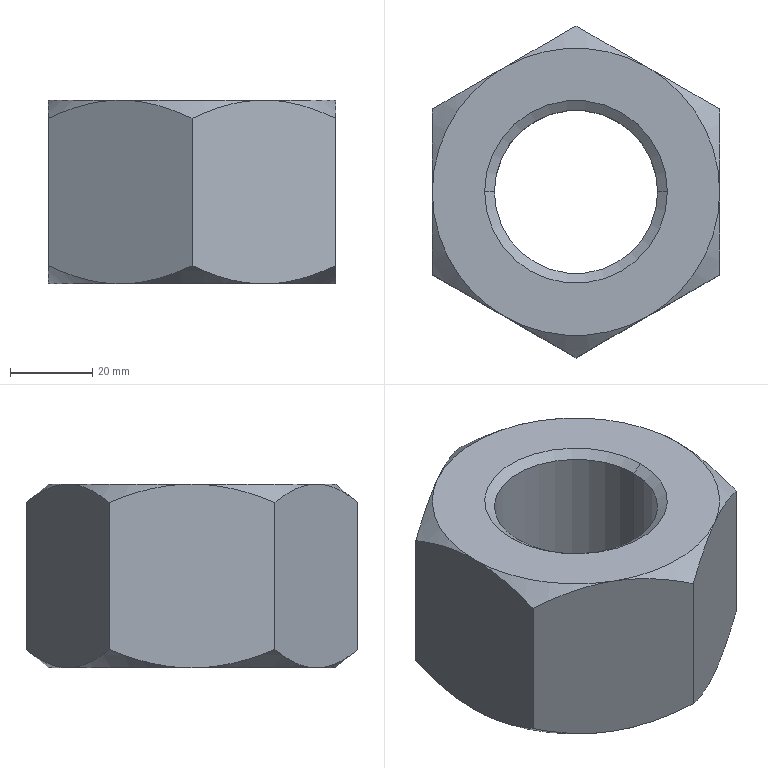Part | SolidWorks | features RevCut 4, Extrusion 1, LPattern 1 | 1 solid | 28 faces | box 69.85 x 80.656 x 44.679 mm | volume 131935 mm3 | cone 16 | plane 8 | cylinder 4 | commonest cylinder face diameters 39.688 x2 44.45 x2
STEP:
#1=CARTESIAN_POINT('',(0.875,0.,-1.759));
#2=VERTEX_POINT('',#1);
#3=CARTESIAN_POINT('',(-0.875,0.,-1.759));
#4=VERTEX_POINT('',#3);
#5=CARTESIAN_POINT('',(0.,0.,-1.759));
#6=DIRECTION('',(0.,0.,-1.));
#7=DIRECTION('',(1.,0.,0.));
#8=AXIS2_PLACEMENT_3D('',#5,#6,#7);
#9=CIRCLE('',#8,0.875);
#10=EDGE_CURVE('',#2,#4,#9,.T.);
#11=ORIENTED_EDGE('',*,*,#10,.T.);
#12=CARTESIAN_POINT('',(-0.875,0.,-1.758));
#13=VERTEX_POINT('',#12);
#14=CARTESIAN_POINT('',(-0.875,0.,-0.9857));
#15=DIRECTION('',(0.,0.,1.));
#16=VECTOR('',#15,39.37);
#17=LINE('',#14,#16);
#18=EDGE_CURVE('',#4,#13,#17,.T.);
#19=ORIENTED_EDGE('',*,*,#18,.T.);
#20=CARTESIAN_POINT('',(0.875,0.,-1.758));
#21=VERTEX_POINT('',#20);
#22=CARTESIAN_POINT('',(0.,0.,-1.758));
#23=DIRECTION('',(0.,0.,1.));
#24=DIRECTION('',(1.,0.,0.));
#25=AXIS2_PLACEMENT_3D('',#22,#23,#24);
#26=CIRCLE('',#25,0.875);
#27=EDGE_CURVE('',#13,#21,#26,.T.);
#28=ORIENTED_EDGE('',*,*,#27,.T.);
#29=CARTESIAN_POINT('',(0.875,0.,-0.9857));
#30=DIRECTION('',(0.,0.,1.));
#31=VECTOR('',#30,39.37);
#32=LINE('',#29,#31);
#33=EDGE_CURVE('',#2,#21,#32,.T.);
#34=ORIENTED_EDGE('',*,*,#33,.F.);
#35=EDGE_LOOP('',(#11,#19,#28,#34));
#36=FACE_OUTER_BOUND('',#35,.T.);
#37=CARTESIAN_POINT('',(0.,0.,-0.9857));
#38=DIRECTION('',(0.,0.,1.));
#39=DIRECTION('',(1.,0.,0.));
#40=AXIS2_PLACEMENT_3D('',#37,#38,#39);
#41=CYLINDRICAL_SURFACE('',#40,0.875);
#42=ADVANCED_FACE('',(#36),#41,.F.);
#43=CARTESIAN_POINT('',(-0.7812,0.,-1.692));
#44=VERTEX_POINT('',#43);
#45=CARTESIAN_POINT('',(0.7812,0.,-1.692));
#46=VERTEX_POINT('',#45);
#47=CARTESIAN_POINT('',(0.,0.,-1.692));
#48=DIRECTION('',(0.,0.,1.));
#49=DIRECTION('',(-1.,0.,0.));
#50=AXIS2_PLACEMENT_3D('',#47,#48,#49);
#51=CIRCLE('',#50,0.7812);
#52=EDGE_CURVE('',#44,#46,#51,.T.);
#53=ORIENTED_EDGE('',*,*,#52,.T.);
#54=CARTESIAN_POINT('',(0.875,0.,-1.758));
#55=DIRECTION('',(0.8192,0.,-0.5736));
#56=VECTOR('',#55,39.37);
#57=LINE('',#54,#56);
#58=EDGE_CURVE('',#46,#21,#57,.T.);
#59=ORIENTED_EDGE('',*,*,#58,.T.);
#60=ORIENTED_EDGE('',*,*,#27,.F.);
#61=CARTESIAN_POINT('',(-0.875,0.,-1.758));
#62=DIRECTION('',(-0.8192,0.,-0.5736));
#63=VECTOR('',#62,39.37);
#64=LINE('',#61,#63);
#65=EDGE_CURVE('',#44,#13,#64,.T.);
#66=ORIENTED_EDGE('',*,*,#65,.F.);
#67=EDGE_LOOP('',(#53,#59,#60,#66));
#68=FACE_OUTER_BOUND('',#67,.T.);
#69=CARTESIAN_POINT('',(0.,0.,-1.758));
#70=DIRECTION('',(0.,0.,-1.));
#71=DIRECTION('',(-1.,0.,0.));
#72=AXIS2_PLACEMENT_3D('',#69,#70,#71);
#73=CONICAL_SURFACE('',#72,0.875,0.9599);
#74=ADVANCED_FACE('',(#68),#73,.F.);
#75=CARTESIAN_POINT('',(0.7812,0.,-0.06564));
#76=VERTEX_POINT('',#75);
#77=CARTESIAN_POINT('',(-0.7812,0.,-0.06564));
#78=VERTEX_POINT('',#77);
#79=CARTESIAN_POINT('',(0.,0.,-0.06564));
#80=DIRECTION('',(0.,0.,-1.));
#81=DIRECTION('',(1.,0.,0.));
#82=AXIS2_PLACEMENT_3D('',#79,#80,#81);
#83=CIRCLE('',#82,0.7812);
#84=EDGE_CURVE('',#76,#78,#83,.T.);
#85=ORIENTED_EDGE('',*,*,#84,.T.);
#86=CARTESIAN_POINT('',(-0.875,0.,0.));
#87=VERTEX_POINT('',#86);
#88=CARTESIAN_POINT('',(-0.7719,0.,-0.07221));
#89=DIRECTION('',(-0.8192,0.,0.5736));
#90=VECTOR('',#89,39.37);
#91=LINE('',#88,#90);
#92=EDGE_CURVE('',#78,#87,#91,.T.);
#93=ORIENTED_EDGE('',*,*,#92,.T.);
#94=CARTESIAN_POINT('',(0.875,0.,0.));
#95=VERTEX_POINT('',#94);
#96=CARTESIAN_POINT('',(0.,0.,0.));
#97=DIRECTION('',(0.,0.,1.));
#98=DIRECTION('',(1.,0.,0.));
#99=AXIS2_PLACEMENT_3D('',#96,#97,#98);
#100=CIRCLE('',#99,0.875);
#101=EDGE_CURVE('',#87,#95,#100,.T.);
#102=ORIENTED_EDGE('',*,*,#101,.T.);
#103=CARTESIAN_POINT('',(0.7719,0.,-0.07221));
#104=DIRECTION('',(0.8192,0.,0.5736));
#105=VECTOR('',#104,39.37);
#106=LINE('',#103,#105);
#107=EDGE_CURVE('',#76,#95,#106,.T.);
#108=ORIENTED_EDGE('',*,*,#107,.F.);
#109=EDGE_LOOP('',(#85,#93,#102,#108));
#110=FACE_OUTER_BOUND('',#109,.T.);
#111=CARTESIAN_POINT('',(0.,0.,-0.07221));
#112=DIRECTION('',(0.,0.,1.));
#113=DIRECTION('',(1.,0.,0.));
#114=AXIS2_PLACEMENT_3D('',#111,#112,#113);
#115=CONICAL_SURFACE('',#114,0.7719,0.9599);
#116=ADVANCED_FACE('',(#110),#115,.F.);
#117=ORIENTED_EDGE('',*,*,#52,.F.);
#118=CARTESIAN_POINT('',(-0.7812,0.,-1.759));
#119=DIRECTION('',(0.,0.,1.));
#120=VECTOR('',#119,39.37);
#121=LINE('',#118,#120);
#122=EDGE_CURVE('',#44,#78,#121,.T.);
#123=ORIENTED_EDGE('',*,*,#122,.T.);
#124=ORIENTED_EDGE('',*,*,#84,.F.);
#125=CARTESIAN_POINT('',(0.7812,0.,-1.759));
#126=DIRECTION('',(0.,0.,1.));
#127=VECTOR('',#126,39.37);
#128=LINE('',#125,#127);
#129=EDGE_CURVE('',#46,#76,#128,.T.);
#130=ORIENTED_EDGE('',*,*,#129,.F.);
#131=EDGE_LOOP('',(#117,#123,#124,#130));
#132=FACE_OUTER_BOUND('',#131,.T.);
#133=CARTESIAN_POINT('',(0.,0.,-1.759));
#134=DIRECTION('',(0.,0.,1.));
#135=DIRECTION('',(1.,0.,0.));
#136=AXIS2_PLACEMENT_3D('',#133,#134,#135);
#137=CYLINDRICAL_SURFACE('',#136,0.7812);
#138=ADVANCED_FACE('',(#132),#137,.F.);
#139=ORIENTED_EDGE('',*,*,#122,.F.);
#140=CARTESIAN_POINT('',(0.,0.,-1.692));
#141=DIRECTION('',(0.,0.,1.));
#142=DIRECTION('',(-1.,0.,0.));
#143=AXIS2_PLACEMENT_3D('',#140,#141,#142);
#144=CIRCLE('',#143,0.7812);
#145=EDGE_CURVE('',#46,#44,#144,.T.);
#146=ORIENTED_EDGE('',*,*,#145,.F.);
#147=ORIENTED_EDGE('',*,*,#129,.T.);
#148=CARTESIAN_POINT('',(0.,0.,-0.06564));
#149=DIRECTION('',(0.,0.,-1.));
#150=DIRECTION('',(1.,0.,0.));
#151=AXIS2_PLACEMENT_3D('',#148,#149,#150);
#152=CIRCLE('',#151,0.7812);
#153=EDGE_CURVE('',#78,#76,#152,.T.);
#154=ORIENTED_EDGE('',*,*,#153,.F.);
#155=EDGE_LOOP('',(#139,#146,#147,#154));
#156=FACE_OUTER_BOUND('',#155,.T.);
#157=CARTESIAN_POINT('',(0.,0.,-1.759));
#158=DIRECTION('',(0.,0.,1.));
#159=DIRECTION('',(1.,0.,0.));
#160=AXIS2_PLACEMENT_3D('',#157,#158,#159);
#161=CYLINDRICAL_SURFACE('',#160,0.7812);
#162=ADVANCED_FACE('',(#156),#161,.F.);
#163=CARTESIAN_POINT('',(-1.375,0.7939,-1.584));
#164=VERTEX_POINT('',#163);
#165=CARTESIAN_POINT('',(-1.375,0.7939,-0.175));
#166=VERTEX_POINT('',#165);
#167=CARTESIAN_POINT('',(-1.375,0.7939,-1.759));
#168=DIRECTION('',(0.,0.,1.));
#169=VECTOR('',#168,39.37);
#170=LINE('',#167,#169);
#171=EDGE_CURVE('',#164,#166,#170,.T.);
#172=ORIENTED_EDGE('',*,*,#171,.T.);
#173=CARTESIAN_POINT('',(-0.6875,1.191,0.));
#174=VERTEX_POINT('',#173);
#175=CARTESIAN_POINT('',(-1.375,0.7939,-0.175));
#176=CARTESIAN_POINT('',(-1.265,0.8572,-0.1229));
#177=CARTESIAN_POINT('',(-1.154,0.9217,-0.07908));
#178=CARTESIAN_POINT('',(-0.9819,1.021,-0.0329));
#179=CARTESIAN_POINT('',(-0.924,1.054,-0.02077));
#180=CARTESIAN_POINT('',(-0.8358,1.105,-0.008404));
#181=CARTESIAN_POINT('',(-0.8061,1.122,-0.005249));
#182=CARTESIAN_POINT('',(-0.7466,1.157,-0.001043));
#183=CARTESIAN_POINT('',(-0.717,1.174,0.));
#184=CARTESIAN_POINT('',(-0.6875,1.191,0.));
#185=B_SPLINE_CURVE_WITH_KNOTS('',3,(#175,#176,#177,#178,#179,#180,#181,#182,#183,#184),.UNSPECIFIED.,.F.,.F.,(4,2,2,2,4),(0.000000247,0.01034,0.01551,0.01809,0.02068),.UNSPECIFIED.);
#186=EDGE_CURVE('',#166,#174,#185,.T.);
#187=ORIENTED_EDGE('',*,*,#186,.T.);
#188=CARTESIAN_POINT('',(0.,1.588,-0.175));
#189=VERTEX_POINT('',#188);
#190=CARTESIAN_POINT('',(-0.6875,1.191,0.));
#191=CARTESIAN_POINT('',(-0.6284,1.225,0.));
#192=CARTESIAN_POINT('',(-0.5697,1.259,-0.004204));
#193=CARTESIAN_POINT('',(-0.4533,1.326,-0.02037));
#194=CARTESIAN_POINT('',(-0.3956,1.359,-0.03232));
#195=CARTESIAN_POINT('',(-0.2809,1.426,-0.06299));
#196=CARTESIAN_POINT('',(-0.2239,1.458,-0.08172));
#197=CARTESIAN_POINT('',(-0.1108,1.524,-0.1247));
#198=CARTESIAN_POINT('',(-0.05506,1.556,-0.1488));
#199=CARTESIAN_POINT('',(0.,1.588,-0.175));
#200=B_SPLINE_CURVE_WITH_KNOTS('',3,(#190,#191,#192,#193,#194,#195,#196,#197,#198,#199),.UNSPECIFIED.,.F.,.F.,(4,2,2,2,4),(0.02068,0.02586,0.03104,0.03622,0.0414),.UNSPECIFIED.);
#201=EDGE_CURVE('',#174,#189,#200,.T.);
#202=ORIENTED_EDGE('',*,*,#201,.T.);
#203=CARTESIAN_POINT('',(0.,1.588,-1.584));
#204=VERTEX_POINT('',#203);
#205=CARTESIAN_POINT('',(0.,1.588,-1.759));
#206=DIRECTION('',(0.,0.,1.));
#207=VECTOR('',#206,39.37);
#208=LINE('',#205,#207);
#209=EDGE_CURVE('',#204,#189,#208,.T.);
#210=ORIENTED_EDGE('',*,*,#209,.F.);
#211=CARTESIAN_POINT('',(-0.6875,1.191,-1.759));
#212=VERTEX_POINT('',#211);
#213=CARTESIAN_POINT('',(-0.6875,1.191,-1.759));
#214=CARTESIAN_POINT('',(-0.6284,1.225,-1.759));
#215=CARTESIAN_POINT('',(-0.5697,1.259,-1.755));
#216=CARTESIAN_POINT('',(-0.4533,1.326,-1.739));
#217=CARTESIAN_POINT('',(-0.3956,1.359,-1.727));
#218=CARTESIAN_POINT('',(-0.2809,1.426,-1.696));
#219=CARTESIAN_POINT('',(-0.2239,1.458,-1.677));
#220=CARTESIAN_POINT('',(-0.1108,1.524,-1.634));
#221=CARTESIAN_POINT('',(-0.05506,1.556,-1.61));
#222=CARTESIAN_POINT('',(0.,1.588,-1.584));
#223=B_SPLINE_CURVE_WITH_KNOTS('',3,(#213,#214,#215,#216,#217,#218,#219,#220,#221,#222),.UNSPECIFIED.,.F.,.F.,(4,2,2,2,4),(0.02068,0.02586,0.03104,0.03622,0.0414),.UNSPECIFIED.);
#224=EDGE_CURVE('',#212,#204,#223,.T.);
#225=ORIENTED_EDGE('',*,*,#224,.F.);
#226=CARTESIAN_POINT('',(-1.375,0.7939,-1.584));
#227=CARTESIAN_POINT('',(-1.265,0.8572,-1.636));
#228=CARTESIAN_POINT('',(-1.154,0.9217,-1.68));
#229=CARTESIAN_POINT('',(-0.9819,1.021,-1.726));
#230=CARTESIAN_POINT('',(-0.924,1.054,-1.738));
#231=CARTESIAN_POINT('',(-0.8358,1.105,-1.751));
#232=CARTESIAN_POINT('',(-0.8061,1.122,-1.754));
#233=CARTESIAN_POINT('',(-0.7466,1.157,-1.758));
#234=CARTESIAN_POINT('',(-0.717,1.174,-1.759));
#235=CARTESIAN_POINT('',(-0.6875,1.191,-1.759));
#236=B_SPLINE_CURVE_WITH_KNOTS('',3,(#226,#227,#228,#229,#230,#231,#232,#233,#234,#235),.UNSPECIFIED.,.F.,.F.,(4,2,2,2,4),(0.000000247,0.01034,0.01551,0.01809,0.02068),.UNSPECIFIED.);
#237=EDGE_CURVE('',#164,#212,#236,.T.);
#238=ORIENTED_EDGE('',*,*,#237,.F.);
#239=EDGE_LOOP('',(#172,#187,#202,#210,#225,#238));
#240=FACE_OUTER_BOUND('',#239,.T.);
#241=CARTESIAN_POINT('',(0.,1.588,-1.759));
#242=DIRECTION('',(-0.5,0.866,0.));
#243=DIRECTION('',(-0.866,-0.5,0.));
#244=AXIS2_PLACEMENT_3D('',#241,#242,#243);
#245=PLANE('',#244);
#246=ADVANCED_FACE('',(#240),#245,.T.);
#247=ORIENTED_EDGE('',*,*,#209,.T.);
#248=CARTESIAN_POINT('',(0.6875,1.191,0.));
#249=VERTEX_POINT('',#248);
#250=CARTESIAN_POINT('',(0.,1.588,-0.175));
#251=CARTESIAN_POINT('',(0.1098,1.524,-0.1229));
#252=CARTESIAN_POINT('',(0.2214,1.46,-0.07908));
#253=CARTESIAN_POINT('',(0.3931,1.361,-0.0329));
#254=CARTESIAN_POINT('',(0.451,1.327,-0.02077));
#255=CARTESIAN_POINT('',(0.5392,1.276,-0.008404));
#256=CARTESIAN_POINT('',(0.5689,1.259,-0.005249));
#257=CARTESIAN_POINT('',(0.6284,1.225,-0.001043));
#258=CARTESIAN_POINT('',(0.658,1.208,0.));
#259=CARTESIAN_POINT('',(0.6875,1.191,0.));
#260=B_SPLINE_CURVE_WITH_KNOTS('',3,(#250,#251,#252,#253,#254,#255,#256,#257,#258,#259),.UNSPECIFIED.,.F.,.F.,(4,2,2,2,4),(0.000000247,0.01034,0.01551,0.01809,0.02068),.UNSPECIFIED.);
#261=EDGE_CURVE('',#189,#249,#260,.T.);
#262=ORIENTED_EDGE('',*,*,#261,.T.);
#263=CARTESIAN_POINT('',(1.375,0.7939,-0.175));
#264=VERTEX_POINT('',#263);
#265=CARTESIAN_POINT('',(0.6875,1.191,0.));
#266=CARTESIAN_POINT('',(0.7466,1.157,0.));
#267=CARTESIAN_POINT('',(0.8053,1.123,-0.004204));
#268=CARTESIAN_POINT('',(0.9217,1.056,-0.02037));
#269=CARTESIAN_POINT('',(0.9794,1.022,-0.03232));
#270=CARTESIAN_POINT('',(1.094,0.956,-0.06299));
#271=CARTESIAN_POINT('',(1.151,0.9231,-0.08172));
#272=CARTESIAN_POINT('',(1.264,0.8578,-0.1247));
#273=CARTESIAN_POINT('',(1.32,0.8256,-0.1488));
#274=CARTESIAN_POINT('',(1.375,0.7939,-0.175));
#275=B_SPLINE_CURVE_WITH_KNOTS('',3,(#265,#266,#267,#268,#269,#270,#271,#272,#273,#274),.UNSPECIFIED.,.F.,.F.,(4,2,2,2,4),(0.02068,0.02586,0.03104,0.03622,0.0414),.UNSPECIFIED.);
#276=EDGE_CURVE('',#249,#264,#275,.T.);
#277=ORIENTED_EDGE('',*,*,#276,.T.);
#278=CARTESIAN_POINT('',(1.375,0.7939,-1.584));
#279=VERTEX_POINT('',#278);
#280=CARTESIAN_POINT('',(1.375,0.7939,-1.759));
#281=DIRECTION('',(0.,0.,1.));
#282=VECTOR('',#281,39.37);
#283=LINE('',#280,#282);
#284=EDGE_CURVE('',#279,#264,#283,.T.);
#285=ORIENTED_EDGE('',*,*,#284,.F.);
#286=CARTESIAN_POINT('',(0.6875,1.191,-1.759));
#287=VERTEX_POINT('',#286);
#288=CARTESIAN_POINT('',(0.6875,1.191,-1.759));
#289=CARTESIAN_POINT('',(0.7466,1.157,-1.759));
#290=CARTESIAN_POINT('',(0.8053,1.123,-1.755));
#291=CARTESIAN_POINT('',(0.9217,1.056,-1.739));
#292=CARTESIAN_POINT('',(0.9794,1.022,-1.727));
#293=CARTESIAN_POINT('',(1.094,0.956,-1.696));
#294=CARTESIAN_POINT('',(1.151,0.9231,-1.677));
#295=CARTESIAN_POINT('',(1.264,0.8578,-1.634));
#296=CARTESIAN_POINT('',(1.32,0.8256,-1.61));
#297=CARTESIAN_POINT('',(1.375,0.7939,-1.584));
#298=B_SPLINE_CURVE_WITH_KNOTS('',3,(#288,#289,#290,#291,#292,#293,#294,#295,#296,#297),.UNSPECIFIED.,.F.,.F.,(4,2,2,2,4),(0.02068,0.02586,0.03104,0.03622,0.0414),.UNSPECIFIED.);
#299=EDGE_CURVE('',#287,#279,#298,.T.);
#300=ORIENTED_EDGE('',*,*,#299,.F.);
#301=CARTESIAN_POINT('',(0.,1.588,-1.584));
#302=CARTESIAN_POINT('',(0.1098,1.524,-1.636));
#303=CARTESIAN_POINT('',(0.2214,1.46,-1.68));
#304=CARTESIAN_POINT('',(0.3931,1.361,-1.726));
#305=CARTESIAN_POINT('',(0.451,1.327,-1.738));
#306=CARTESIAN_POINT('',(0.5392,1.276,-1.751));
#307=CARTESIAN_POINT('',(0.5689,1.259,-1.754));
#308=CARTESIAN_POINT('',(0.6284,1.225,-1.758));
#309=CARTESIAN_POINT('',(0.658,1.208,-1.759));
#310=CARTESIAN_POINT('',(0.6875,1.191,-1.759));
#311=B_SPLINE_CURVE_WITH_KNOTS('',3,(#301,#302,#303,#304,#305,#306,#307,#308,#309,#310),.UNSPECIFIED.,.F.,.F.,(4,2,2,2,4),(0.000000247,0.01034,0.01551,0.01809,0.02068),.UNSPECIFIED.);
#312=EDGE_CURVE('',#204,#287,#311,.T.);
#313=ORIENTED_EDGE('',*,*,#312,.F.);
#314=EDGE_LOOP('',(#247,#262,#277,#285,#300,#313));
#315=FACE_OUTER_BOUND('',#314,.T.);
#316=CARTESIAN_POINT('',(1.375,0.7939,-1.759));
#317=DIRECTION('',(0.5,0.866,0.));
#318=DIRECTION('',(-0.866,0.5,0.));
#319=AXIS2_PLACEMENT_3D('',#316,#317,#318);
#320=PLANE('',#319);
#321=ADVANCED_FACE('',(#315),#320,.T.);
#322=CARTESIAN_POINT('',(1.375,-0.7939,-0.175));
#323=VERTEX_POINT('',#322);
#324=CARTESIAN_POINT('',(1.375,0.,0.));
#325=VERTEX_POINT('',#324);
#326=CARTESIAN_POINT('',(1.375,-0.7939,-0.175));
#327=CARTESIAN_POINT('',(1.375,-0.7309,-0.1491));
#328=CARTESIAN_POINT('',(1.375,-0.6669,-0.1251));
#329=CARTESIAN_POINT('',(1.375,-0.5363,-0.08201));
#330=CARTESIAN_POINT('',(1.375,-0.4704,-0.06323));
#331=CARTESIAN_POINT('',(1.375,-0.3379,-0.03248));
#332=CARTESIAN_POINT('',(1.375,-0.2711,-0.02047));
#333=CARTESIAN_POINT('',(1.375,-0.1364,-0.004232));
#334=CARTESIAN_POINT('',(1.375,-0.06852,0.));
#335=CARTESIAN_POINT('',(1.375,0.,0.));
#336=B_SPLINE_CURVE_WITH_KNOTS('',3,(#326,#327,#328,#329,#330,#331,#332,#333,#334,#335),.UNSPECIFIED.,.F.,.F.,(4,2,2,2,4),(0.02901,0.03418,0.03934,0.04451,0.04968),.UNSPECIFIED.);
#337=EDGE_CURVE('',#323,#325,#336,.T.);
#338=ORIENTED_EDGE('',*,*,#337,.F.);
#339=CARTESIAN_POINT('',(1.375,-0.7939,-1.584));
#340=VERTEX_POINT('',#339);
#341=CARTESIAN_POINT('',(1.375,-0.7939,-1.759));
#342=DIRECTION('',(0.,0.,1.));
#343=VECTOR('',#342,39.37);
#344=LINE('',#341,#343);
#345=EDGE_CURVE('',#340,#323,#344,.T.);
#346=ORIENTED_EDGE('',*,*,#345,.F.);
#347=CARTESIAN_POINT('',(1.375,0.,-1.759));
#348=VERTEX_POINT('',#347);
#349=CARTESIAN_POINT('',(1.375,-0.7939,-1.584));
#350=CARTESIAN_POINT('',(1.375,-0.7309,-1.61));
#351=CARTESIAN_POINT('',(1.375,-0.6669,-1.634));
#352=CARTESIAN_POINT('',(1.375,-0.5363,-1.677));
#353=CARTESIAN_POINT('',(1.375,-0.4704,-1.696));
#354=CARTESIAN_POINT('',(1.375,-0.3379,-1.727));
#355=CARTESIAN_POINT('',(1.375,-0.2711,-1.739));
#356=CARTESIAN_POINT('',(1.375,-0.1364,-1.755));
#357=CARTESIAN_POINT('',(1.375,-0.06852,-1.759));
#358=CARTESIAN_POINT('',(1.375,0.,-1.759));
#359=B_SPLINE_CURVE_WITH_KNOTS('',3,(#349,#350,#351,#352,#353,#354,#355,#356,#357,#358),.UNSPECIFIED.,.F.,.F.,(4,2,2,2,4),(0.02901,0.03418,0.03934,0.04451,0.04968),.UNSPECIFIED.);
#360=EDGE_CURVE('',#340,#348,#359,.T.);
#361=ORIENTED_EDGE('',*,*,#360,.T.);
#362=CARTESIAN_POINT('',(1.375,0.,-1.759));
#363=CARTESIAN_POINT('',(1.375,0.03412,-1.759));
#364=CARTESIAN_POINT('',(1.375,0.0685,-1.758));
#365=CARTESIAN_POINT('',(1.375,0.1371,-1.754));
#366=CARTESIAN_POINT('',(1.375,0.1711,-1.751));
#367=CARTESIAN_POINT('',(1.375,0.2726,-1.738));
#368=CARTESIAN_POINT('',(1.375,0.3394,-1.726));
#369=CARTESIAN_POINT('',(1.375,0.4716,-1.695));
#370=CARTESIAN_POINT('',(1.375,0.537,-1.677));
#371=CARTESIAN_POINT('',(1.375,0.6665,-1.634));
#372=CARTESIAN_POINT('',(1.375,0.7309,-1.61));
#373=CARTESIAN_POINT('',(1.375,0.7939,-1.584));
#374=B_SPLINE_CURVE_WITH_KNOTS('',3,(#362,#363,#364,#365,#366,#367,#368,#369,#370,#371,#372,#373),.UNSPECIFIED.,.F.,.F.,(4,2,2,2,2,4),(0.04968,0.05226,0.05483,0.05998,0.06513,0.07027),.UNSPECIFIED.);
#375=EDGE_CURVE('',#348,#279,#374,.T.);
#376=ORIENTED_EDGE('',*,*,#375,.T.);
#377=ORIENTED_EDGE('',*,*,#284,.T.);
#378=CARTESIAN_POINT('',(1.375,0.,0.));
#379=CARTESIAN_POINT('',(1.375,0.03412,0.));
#380=CARTESIAN_POINT('',(1.375,0.0685,-0.001054));
#381=CARTESIAN_POINT('',(1.375,0.1371,-0.005258));
#382=CARTESIAN_POINT('',(1.375,0.1711,-0.008393));
#383=CARTESIAN_POINT('',(1.375,0.2726,-0.0207));
#384=CARTESIAN_POINT('',(1.375,0.3394,-0.03279));
#385=CARTESIAN_POINT('',(1.375,0.4716,-0.06355));
#386=CARTESIAN_POINT('',(1.375,0.537,-0.08222));
#387=CARTESIAN_POINT('',(1.375,0.6665,-0.1249));
#388=CARTESIAN_POINT('',(1.375,0.7309,-0.1491));
#389=CARTESIAN_POINT('',(1.375,0.7939,-0.175));
#390=B_SPLINE_CURVE_WITH_KNOTS('',3,(#378,#379,#380,#381,#382,#383,#384,#385,#386,#387,#388,#389),.UNSPECIFIED.,.F.,.F.,(4,2,2,2,2,4),(0.04968,0.05226,0.05483,0.05998,0.06513,0.07027),.UNSPECIFIED.);
#391=EDGE_CURVE('',#325,#264,#390,.T.);
#392=ORIENTED_EDGE('',*,*,#391,.F.);
#393=EDGE_LOOP('',(#338,#346,#361,#376,#377,#392));
#394=FACE_OUTER_BOUND('',#393,.T.);
#395=CARTESIAN_POINT('',(1.375,0.7939,-1.759));
#396=DIRECTION('',(-1.,0.,0.));
#397=DIRECTION('',(0.,0.,1.));
#398=AXIS2_PLACEMENT_3D('',#395,#396,#397);
#399=PLANE('',#398);
#400=ADVANCED_FACE('',(#394),#399,.F.);
#401=ORIENTED_EDGE('',*,*,#345,.T.);
#402=CARTESIAN_POINT('',(0.6875,-1.191,0.));
#403=VERTEX_POINT('',#402);
#404=CARTESIAN_POINT('',(1.375,-0.7939,-0.175));
#405=CARTESIAN_POINT('',(1.265,-0.8572,-0.1229));
#406=CARTESIAN_POINT('',(1.154,-0.9217,-0.07908));
#407=CARTESIAN_POINT('',(0.9819,-1.021,-0.0329));
#408=CARTESIAN_POINT('',(0.924,-1.054,-0.02077));
#409=CARTESIAN_POINT('',(0.8358,-1.105,-0.008404));
#410=CARTESIAN_POINT('',(0.8061,-1.122,-0.005249));
#411=CARTESIAN_POINT('',(0.7466,-1.157,-0.001043));
#412=CARTESIAN_POINT('',(0.717,-1.174,0.));
#413=CARTESIAN_POINT('',(0.6875,-1.191,0.));
#414=B_SPLINE_CURVE_WITH_KNOTS('',3,(#404,#405,#406,#407,#408,#409,#410,#411,#412,#413),.UNSPECIFIED.,.F.,.F.,(4,2,2,2,4),(0.000000247,0.01034,0.01551,0.01809,0.02068),.UNSPECIFIED.);
#415=EDGE_CURVE('',#323,#403,#414,.T.);
#416=ORIENTED_EDGE('',*,*,#415,.T.);
#417=CARTESIAN_POINT('',(0.,-1.588,-0.175));
#418=VERTEX_POINT('',#417);
#419=CARTESIAN_POINT('',(0.6875,-1.191,0.));
#420=CARTESIAN_POINT('',(0.6284,-1.225,0.));
#421=CARTESIAN_POINT('',(0.5697,-1.259,-0.004204));
#422=CARTESIAN_POINT('',(0.4533,-1.326,-0.02037));
#423=CARTESIAN_POINT('',(0.3956,-1.359,-0.03232));
#424=CARTESIAN_POINT('',(0.2809,-1.426,-0.06299));
#425=CARTESIAN_POINT('',(0.2239,-1.458,-0.08172));
#426=CARTESIAN_POINT('',(0.1108,-1.524,-0.1247));
#427=CARTESIAN_POINT('',(0.05506,-1.556,-0.1488));
#428=CARTESIAN_POINT('',(0.,-1.588,-0.175));
#429=B_SPLINE_CURVE_WITH_KNOTS('',3,(#419,#420,#421,#422,#423,#424,#425,#426,#427,#428),.UNSPECIFIED.,.F.,.F.,(4,2,2,2,4),(0.02068,0.02586,0.03104,0.03622,0.0414),.UNSPECIFIED.);
#430=EDGE_CURVE('',#403,#418,#429,.T.);
#431=ORIENTED_EDGE('',*,*,#430,.T.);
#432=CARTESIAN_POINT('',(0.,-1.588,-1.584));
#433=VERTEX_POINT('',#432);
#434=CARTESIAN_POINT('',(0.,-1.588,-1.759));
#435=DIRECTION('',(0.,0.,1.));
#436=VECTOR('',#435,39.37);
#437=LINE('',#434,#436);
#438=EDGE_CURVE('',#433,#418,#437,.T.);
#439=ORIENTED_EDGE('',*,*,#438,.F.);
#440=CARTESIAN_POINT('',(0.6875,-1.191,-1.759));
#441=VERTEX_POINT('',#440);
#442=CARTESIAN_POINT('',(0.6875,-1.191,-1.759));
#443=CARTESIAN_POINT('',(0.6284,-1.225,-1.759));
#444=CARTESIAN_POINT('',(0.5697,-1.259,-1.755));
#445=CARTESIAN_POINT('',(0.4533,-1.326,-1.739));
#446=CARTESIAN_POINT('',(0.3956,-1.359,-1.727));
#447=CARTESIAN_POINT('',(0.2809,-1.426,-1.696));
#448=CARTESIAN_POINT('',(0.2239,-1.458,-1.677));
#449=CARTESIAN_POINT('',(0.1108,-1.524,-1.634));
#450=CARTESIAN_POINT('',(0.05506,-1.556,-1.61));
#451=CARTESIAN_POINT('',(0.,-1.588,-1.584));
#452=B_SPLINE_CURVE_WITH_KNOTS('',3,(#442,#443,#444,#445,#446,#447,#448,#449,#450,#451),.UNSPECIFIED.,.F.,.F.,(4,2,2,2,4),(0.02068,0.02586,0.03104,0.03622,0.0414),.UNSPECIFIED.);
#453=EDGE_CURVE('',#441,#433,#452,.T.);
#454=ORIENTED_EDGE('',*,*,#453,.F.);
#455=CARTESIAN_POINT('',(1.375,-0.7939,-1.584));
#456=CARTESIAN_POINT('',(1.265,-0.8572,-1.636));
#457=CARTESIAN_POINT('',(1.154,-0.9217,-1.68));
#458=CARTESIAN_POINT('',(0.9819,-1.021,-1.726));
#459=CARTESIAN_POINT('',(0.924,-1.054,-1.738));
#460=CARTESIAN_POINT('',(0.8358,-1.105,-1.751));
#461=CARTESIAN_POINT('',(0.8061,-1.122,-1.754));
#462=CARTESIAN_POINT('',(0.7466,-1.157,-1.758));
#463=CARTESIAN_POINT('',(0.717,-1.174,-1.759));
#464=CARTESIAN_POINT('',(0.6875,-1.191,-1.759));
#465=B_SPLINE_CURVE_WITH_KNOTS('',3,(#455,#456,#457,#458,#459,#460,#461,#462,#463,#464),.UNSPECIFIED.,.F.,.F.,(4,2,2,2,4),(0.000000247,0.01034,0.01551,0.01809,0.02068),.UNSPECIFIED.);
#466=EDGE_CURVE('',#340,#441,#465,.T.);
#467=ORIENTED_EDGE('',*,*,#466,.F.);
#468=EDGE_LOOP('',(#401,#416,#431,#439,#454,#467));
#469=FACE_OUTER_BOUND('',#468,.T.);
#470=CARTESIAN_POINT('',(0.,-1.588,-1.759));
#471=DIRECTION('',(0.5,-0.866,0.));
#472=DIRECTION('',(0.866,0.5,0.));
#473=AXIS2_PLACEMENT_3D('',#470,#471,#472);
#474=PLANE('',#473);
#475=ADVANCED_FACE('',(#469),#474,.T.);
#476=ORIENTED_EDGE('',*,*,#438,.T.);
#477=CARTESIAN_POINT('',(-0.6875,-1.191,0.));
#478=VERTEX_POINT('',#477);
#479=CARTESIAN_POINT('',(0.,-1.588,-0.175));
#480=CARTESIAN_POINT('',(-0.1098,-1.524,-0.1229));
#481=CARTESIAN_POINT('',(-0.2214,-1.46,-0.07908));
#482=CARTESIAN_POINT('',(-0.3931,-1.361,-0.0329));
#483=CARTESIAN_POINT('',(-0.451,-1.327,-0.02077));
#484=CARTESIAN_POINT('',(-0.5392,-1.276,-0.008404));
#485=CARTESIAN_POINT('',(-0.5689,-1.259,-0.005249));
#486=CARTESIAN_POINT('',(-0.6284,-1.225,-0.001043));
#487=CARTESIAN_POINT('',(-0.658,-1.208,0.));
#488=CARTESIAN_POINT('',(-0.6875,-1.191,0.));
#489=B_SPLINE_CURVE_WITH_KNOTS('',3,(#479,#480,#481,#482,#483,#484,#485,#486,#487,#488),.UNSPECIFIED.,.F.,.F.,(4,2,2,2,4),(0.000000247,0.01034,0.01551,0.01809,0.02068),.UNSPECIFIED.);
#490=EDGE_CURVE('',#418,#478,#489,.T.);
#491=ORIENTED_EDGE('',*,*,#490,.T.);
#492=CARTESIAN_POINT('',(-1.375,-0.7939,-0.175));
#493=VERTEX_POINT('',#492);
#494=CARTESIAN_POINT('',(-0.6875,-1.191,0.));
#495=CARTESIAN_POINT('',(-0.7466,-1.157,0.));
#496=CARTESIAN_POINT('',(-0.8053,-1.123,-0.004204));
#497=CARTESIAN_POINT('',(-0.9217,-1.056,-0.02037));
#498=CARTESIAN_POINT('',(-0.9794,-1.022,-0.03232));
#499=CARTESIAN_POINT('',(-1.094,-0.956,-0.06299));
#500=CARTESIAN_POINT('',(-1.151,-0.9231,-0.08172));
#501=CARTESIAN_POINT('',(-1.264,-0.8578,-0.1247));
#502=CARTESIAN_POINT('',(-1.32,-0.8256,-0.1488));
#503=CARTESIAN_POINT('',(-1.375,-0.7939,-0.175));
#504=B_SPLINE_CURVE_WITH_KNOTS('',3,(#494,#495,#496,#497,#498,#499,#500,#501,#502,#503),.UNSPECIFIED.,.F.,.F.,(4,2,2,2,4),(0.02068,0.02586,0.03104,0.03622,0.0414),.UNSPECIFIED.);
#505=EDGE_CURVE('',#478,#493,#504,.T.);
#506=ORIENTED_EDGE('',*,*,#505,.T.);
#507=CARTESIAN_POINT('',(-1.375,-0.7939,-1.584));
#508=VERTEX_POINT('',#507);
#509=CARTESIAN_POINT('',(-1.375,-0.7939,-1.759));
#510=DIRECTION('',(0.,0.,1.));
#511=VECTOR('',#510,39.37);
#512=LINE('',#509,#511);
#513=EDGE_CURVE('',#508,#493,#512,.T.);
#514=ORIENTED_EDGE('',*,*,#513,.F.);
#515=CARTESIAN_POINT('',(-0.6875,-1.191,-1.759));
#516=VERTEX_POINT('',#515);
#517=CARTESIAN_POINT('',(-0.6875,-1.191,-1.759));
#518=CARTESIAN_POINT('',(-0.7466,-1.157,-1.759));
#519=CARTESIAN_POINT('',(-0.8053,-1.123,-1.755));
#520=CARTESIAN_POINT('',(-0.9217,-1.056,-1.739));
#521=CARTESIAN_POINT('',(-0.9794,-1.022,-1.727));
#522=CARTESIAN_POINT('',(-1.094,-0.956,-1.696));
#523=CARTESIAN_POINT('',(-1.151,-0.9231,-1.677));
#524=CARTESIAN_POINT('',(-1.264,-0.8578,-1.634));
#525=CARTESIAN_POINT('',(-1.32,-0.8256,-1.61));
#526=CARTESIAN_POINT('',(-1.375,-0.7939,-1.584));
#527=B_SPLINE_CURVE_WITH_KNOTS('',3,(#517,#518,#519,#520,#521,#522,#523,#524,#525,#526),.UNSPECIFIED.,.F.,.F.,(4,2,2,2,4),(0.02068,0.02586,0.03104,0.03622,0.0414),.UNSPECIFIED.);
#528=EDGE_CURVE('',#516,#508,#527,.T.);
#529=ORIENTED_EDGE('',*,*,#528,.F.);
#530=CARTESIAN_POINT('',(0.,-1.588,-1.584));
#531=CARTESIAN_POINT('',(-0.1098,-1.524,-1.636));
#532=CARTESIAN_POINT('',(-0.2214,-1.46,-1.68));
#533=CARTESIAN_POINT('',(-0.3931,-1.361,-1.726));
#534=CARTESIAN_POINT('',(-0.451,-1.327,-1.738));
#535=CARTESIAN_POINT('',(-0.5392,-1.276,-1.751));
#536=CARTESIAN_POINT('',(-0.5689,-1.259,-1.754));
#537=CARTESIAN_POINT('',(-0.6284,-1.225,-1.758));
#538=CARTESIAN_POINT('',(-0.658,-1.208,-1.759));
#539=CARTESIAN_POINT('',(-0.6875,-1.191,-1.759));
#540=B_SPLINE_CURVE_WITH_KNOTS('',3,(#530,#531,#532,#533,#534,#535,#536,#537,#538,#539),.UNSPECIFIED.,.F.,.F.,(4,2,2,2,4),(0.000000247,0.01034,0.01551,0.01809,0.02068),.UNSPECIFIED.);
#541=EDGE_CURVE('',#433,#516,#540,.T.);
#542=ORIENTED_EDGE('',*,*,#541,.F.);
#543=EDGE_LOOP('',(#476,#491,#506,#514,#529,#542));
#544=FACE_OUTER_BOUND('',#543,.T.);
#545=CARTESIAN_POINT('',(-1.375,-0.7939,-1.759));
#546=DIRECTION('',(-0.5,-0.866,0.));
#547=DIRECTION('',(0.866,-0.5,0.));
#548=AXIS2_PLACEMENT_3D('',#545,#546,#547);
#549=PLANE('',#548);
#550=ADVANCED_FACE('',(#544),#549,.T.);
#551=ORIENTED_EDGE('',*,*,#513,.T.);
#552=CARTESIAN_POINT('',(-1.375,0.,0.));
#553=VERTEX_POINT('',#552);
#554=CARTESIAN_POINT('',(-1.375,-0.7939,-0.175));
#555=CARTESIAN_POINT('',(-1.375,-0.7309,-0.1491));
#556=CARTESIAN_POINT('',(-1.375,-0.6669,-0.1251));
#557=CARTESIAN_POINT('',(-1.375,-0.5363,-0.08201));
#558=CARTESIAN_POINT('',(-1.375,-0.4704,-0.06323));
#559=CARTESIAN_POINT('',(-1.375,-0.3379,-0.03248));
#560=CARTESIAN_POINT('',(-1.375,-0.2711,-0.02047));
#561=CARTESIAN_POINT('',(-1.375,-0.1364,-0.004232));
#562=CARTESIAN_POINT('',(-1.375,-0.06852,0.));
#563=CARTESIAN_POINT('',(-1.375,0.,0.));
#564=B_SPLINE_CURVE_WITH_KNOTS('',3,(#554,#555,#556,#557,#558,#559,#560,#561,#562,#563),.UNSPECIFIED.,.F.,.F.,(4,2,2,2,4),(0.02901,0.03418,0.03934,0.04451,0.04968),.UNSPECIFIED.);
#565=EDGE_CURVE('',#493,#553,#564,.T.);
#566=ORIENTED_EDGE('',*,*,#565,.T.);
#567=CARTESIAN_POINT('',(-1.375,0.,0.));
#568=CARTESIAN_POINT('',(-1.375,0.03412,0.));
#569=CARTESIAN_POINT('',(-1.375,0.0685,-0.001054));
#570=CARTESIAN_POINT('',(-1.375,0.1371,-0.005258));
#571=CARTESIAN_POINT('',(-1.375,0.1711,-0.008393));
#572=CARTESIAN_POINT('',(-1.375,0.2726,-0.0207));
#573=CARTESIAN_POINT('',(-1.375,0.3394,-0.03279));
#574=CARTESIAN_POINT('',(-1.375,0.4716,-0.06355));
#575=CARTESIAN_POINT('',(-1.375,0.537,-0.08222));
#576=CARTESIAN_POINT('',(-1.375,0.6665,-0.1249));
#577=CARTESIAN_POINT('',(-1.375,0.7309,-0.1491));
#578=CARTESIAN_POINT('',(-1.375,0.7939,-0.175));
#579=B_SPLINE_CURVE_WITH_KNOTS('',3,(#567,#568,#569,#570,#571,#572,#573,#574,#575,#576,#577,#578),.UNSPECIFIED.,.F.,.F.,(4,2,2,2,2,4),(0.04968,0.05226,0.05483,0.05998,0.06513,0.07027),.UNSPECIFIED.);
#580=EDGE_CURVE('',#553,#166,#579,.T.);
#581=ORIENTED_EDGE('',*,*,#580,.T.);
#582=ORIENTED_EDGE('',*,*,#171,.F.);
#583=CARTESIAN_POINT('',(-1.375,0.,-1.759));
#584=VERTEX_POINT('',#583);
#585=CARTESIAN_POINT('',(-1.375,0.,-1.759));
#586=CARTESIAN_POINT('',(-1.375,0.03412,-1.759));
#587=CARTESIAN_POINT('',(-1.375,0.0685,-1.758));
#588=CARTESIAN_POINT('',(-1.375,0.1371,-1.754));
#589=CARTESIAN_POINT('',(-1.375,0.1711,-1.751));
#590=CARTESIAN_POINT('',(-1.375,0.2726,-1.738));
#591=CARTESIAN_POINT('',(-1.375,0.3394,-1.726));
#592=CARTESIAN_POINT('',(-1.375,0.4716,-1.695));
#593=CARTESIAN_POINT('',(-1.375,0.537,-1.677));
#594=CARTESIAN_POINT('',(-1.375,0.6665,-1.634));
#595=CARTESIAN_POINT('',(-1.375,0.7309,-1.61));
#596=CARTESIAN_POINT('',(-1.375,0.7939,-1.584));
#597=B_SPLINE_CURVE_WITH_KNOTS('',3,(#585,#586,#587,#588,#589,#590,#591,#592,#593,#594,#595,#596),.UNSPECIFIED.,.F.,.F.,(4,2,2,2,2,4),(0.04968,0.05226,0.05483,0.05998,0.06513,0.07027),.UNSPECIFIED.);
#598=EDGE_CURVE('',#584,#164,#597,.T.);
#599=ORIENTED_EDGE('',*,*,#598,.F.);
#600=CARTESIAN_POINT('',(-1.375,-0.7939,-1.584));
#601=CARTESIAN_POINT('',(-1.375,-0.7309,-1.61));
#602=CARTESIAN_POINT('',(-1.375,-0.6669,-1.634));
#603=CARTESIAN_POINT('',(-1.375,-0.5363,-1.677));
#604=CARTESIAN_POINT('',(-1.375,-0.4704,-1.696));
#605=CARTESIAN_POINT('',(-1.375,-0.3379,-1.727));
#606=CARTESIAN_POINT('',(-1.375,-0.2711,-1.739));
#607=CARTESIAN_POINT('',(-1.375,-0.1364,-1.755));
#608=CARTESIAN_POINT('',(-1.375,-0.06852,-1.759));
#609=CARTESIAN_POINT('',(-1.375,0.,-1.759));
#610=B_SPLINE_CURVE_WITH_KNOTS('',3,(#600,#601,#602,#603,#604,#605,#606,#607,#608,#609),.UNSPECIFIED.,.F.,.F.,(4,2,2,2,4),(0.02901,0.03418,0.03934,0.04451,0.04968),.UNSPECIFIED.);
#611=EDGE_CURVE('',#508,#584,#610,.T.);
#612=ORIENTED_EDGE('',*,*,#611,.F.);
#613=EDGE_LOOP('',(#551,#566,#581,#582,#599,#612));
#614=FACE_OUTER_BOUND('',#613,.T.);
#615=CARTESIAN_POINT('',(-1.375,0.7939,-1.759));
#616=DIRECTION('',(-1.,0.,0.));
#617=DIRECTION('',(0.,0.,1.));
#618=AXIS2_PLACEMENT_3D('',#615,#616,#617);
#619=PLANE('',#618);
#620=ADVANCED_FACE('',(#614),#619,.T.);
#621=CARTESIAN_POINT('',(0.,0.,0.));
#622=DIRECTION('',(0.,0.,1.));
#623=DIRECTION('',(1.,0.,0.));
#624=AXIS2_PLACEMENT_3D('',#621,#622,#623);
#625=CIRCLE('',#624,0.875);
#626=EDGE_CURVE('',#95,#87,#625,.T.);
#627=ORIENTED_EDGE('',*,*,#626,.F.);
#628=ORIENTED_EDGE('',*,*,#101,.F.);
#629=EDGE_LOOP('',(#627,#628));
#630=FACE_BOUND('',#629,.T.);
#631=CARTESIAN_POINT('',(0.,0.,0.));
#632=DIRECTION('',(0.,0.,1.));
#633=DIRECTION('',(1.,0.,0.));
#634=AXIS2_PLACEMENT_3D('',#631,#632,#633);
#635=CIRCLE('',#634,1.375);
#636=EDGE_CURVE('',#403,#325,#635,.T.);
#637=ORIENTED_EDGE('',*,*,#636,.T.);
#638=CARTESIAN_POINT('',(0.,0.,0.));
#639=DIRECTION('',(0.,0.,1.));
#640=DIRECTION('',(1.,0.,0.));
#641=AXIS2_PLACEMENT_3D('',#638,#639,#640);
#642=CIRCLE('',#641,1.375);
#643=EDGE_CURVE('',#325,#249,#642,.T.);
#644=ORIENTED_EDGE('',*,*,#643,.T.);
#645=CARTESIAN_POINT('',(0.,0.,0.));
#646=DIRECTION('',(0.,0.,1.));
#647=DIRECTION('',(1.,0.,0.));
#648=AXIS2_PLACEMENT_3D('',#645,#646,#647);
#649=CIRCLE('',#648,1.375);
#650=EDGE_CURVE('',#249,#174,#649,.T.);
#651=ORIENTED_EDGE('',*,*,#650,.T.);
#652=CARTESIAN_POINT('',(0.,0.,0.));
#653=DIRECTION('',(0.,0.,1.));
#654=DIRECTION('',(1.,0.,0.));
#655=AXIS2_PLACEMENT_3D('',#652,#653,#654);
#656=CIRCLE('',#655,1.375);
#657=EDGE_CURVE('',#174,#553,#656,.T.);
#658=ORIENTED_EDGE('',*,*,#657,.T.);
#659=CARTESIAN_POINT('',(0.,0.,0.));
#660=DIRECTION('',(0.,0.,1.));
#661=DIRECTION('',(1.,0.,0.));
#662=AXIS2_PLACEMENT_3D('',#659,#660,#661);
#663=CIRCLE('',#662,1.375);
#664=EDGE_CURVE('',#553,#478,#663,.T.);
#665=ORIENTED_EDGE('',*,*,#664,.T.);
#666=CARTESIAN_POINT('',(0.,0.,0.));
#667=DIRECTION('',(0.,0.,1.));
#668=DIRECTION('',(1.,0.,0.));
#669=AXIS2_PLACEMENT_3D('',#666,#667,#668);
#670=CIRCLE('',#669,1.375);
#671=EDGE_CURVE('',#478,#403,#670,.T.);
#672=ORIENTED_EDGE('',*,*,#671,.T.);
#673=EDGE_LOOP('',(#637,#644,#651,#658,#665,#672));
#674=FACE_OUTER_BOUND('',#673,.T.);
#675=CARTESIAN_POINT('',(-1.375,0.7939,0.));
#676=DIRECTION('',(0.,0.,1.));
#677=DIRECTION('',(1.,0.,0.));
#678=AXIS2_PLACEMENT_3D('',#675,#676,#677);
#679=PLANE('',#678);
#680=ADVANCED_FACE('',(#630,#674),#679,.T.);
#681=ORIENTED_EDGE('',*,*,#10,.F.);
#682=CARTESIAN_POINT('',(0.,0.,-1.759));
#683=DIRECTION('',(0.,0.,-1.));
#684=DIRECTION('',(1.,0.,0.));
#685=AXIS2_PLACEMENT_3D('',#682,#683,#684);
#686=CIRCLE('',#685,0.875);
#687=EDGE_CURVE('',#4,#2,#686,.T.);
#688=ORIENTED_EDGE('',*,*,#687,.F.);
#689=EDGE_LOOP('',(#681,#688));
#690=FACE_BOUND('',#689,.T.);
#691=CARTESIAN_POINT('',(0.,0.,-1.759));
#692=DIRECTION('',(0.,0.,1.));
#693=DIRECTION('',(1.,0.,0.));
#694=AXIS2_PLACEMENT_3D('',#691,#692,#693);
#695=CIRCLE('',#694,1.375);
#696=EDGE_CURVE('',#348,#287,#695,.T.);
#697=ORIENTED_EDGE('',*,*,#696,.F.);
#698=CARTESIAN_POINT('',(0.,0.,-1.759));
#699=DIRECTION('',(0.,0.,-1.));
#700=DIRECTION('',(1.,0.,0.));
#701=AXIS2_PLACEMENT_3D('',#698,#699,#700);
#702=CIRCLE('',#701,1.375);
#703=EDGE_CURVE('',#348,#441,#702,.T.);
#704=ORIENTED_EDGE('',*,*,#703,.T.);
#705=CARTESIAN_POINT('',(0.,0.,-1.759));
#706=DIRECTION('',(0.,0.,-1.));
#707=DIRECTION('',(1.,0.,0.));
#708=AXIS2_PLACEMENT_3D('',#705,#706,#707);
#709=CIRCLE('',#708,1.375);
#710=EDGE_CURVE('',#441,#516,#709,.T.);
#711=ORIENTED_EDGE('',*,*,#710,.T.);
#712=CARTESIAN_POINT('',(0.,0.,-1.759));
#713=DIRECTION('',(0.,0.,-1.));
#714=DIRECTION('',(1.,0.,0.));
#715=AXIS2_PLACEMENT_3D('',#712,#713,#714);
#716=CIRCLE('',#715,1.375);
#717=EDGE_CURVE('',#516,#584,#716,.T.);
#718=ORIENTED_EDGE('',*,*,#717,.T.);
#719=CARTESIAN_POINT('',(0.,0.,-1.759));
#720=DIRECTION('',(0.,0.,-1.));
#721=DIRECTION('',(1.,0.,0.));
#722=AXIS2_PLACEMENT_3D('',#719,#720,#721);
#723=CIRCLE('',#722,1.375);
#724=EDGE_CURVE('',#584,#212,#723,.T.);
#725=ORIENTED_EDGE('',*,*,#724,.T.);
#726=CARTESIAN_POINT('',(0.,0.,-1.759));
#727=DIRECTION('',(0.,0.,-1.));
#728=DIRECTION('',(1.,0.,0.));
#729=AXIS2_PLACEMENT_3D('',#726,#727,#728);
#730=CIRCLE('',#729,1.375);
#731=EDGE_CURVE('',#212,#287,#730,.T.);
#732=ORIENTED_EDGE('',*,*,#731,.T.);
#733=EDGE_LOOP('',(#697,#704,#711,#718,#725,#732));
#734=FACE_OUTER_BOUND('',#733,.T.);
#735=CARTESIAN_POINT('',(-1.375,0.7939,-1.759));
#736=DIRECTION('',(0.,0.,1.));
#737=DIRECTION('',(1.,0.,0.));
#738=AXIS2_PLACEMENT_3D('',#735,#736,#737);
#739=PLANE('',#738);
#740=ADVANCED_FACE('',(#690,#734),#739,.F.);
#741=ORIENTED_EDGE('',*,*,#299,.T.);
#742=ORIENTED_EDGE('',*,*,#375,.F.);
#743=ORIENTED_EDGE('',*,*,#696,.T.);
#744=EDGE_LOOP('',(#741,#742,#743));
#745=FACE_OUTER_BOUND('',#744,.T.);
#746=CARTESIAN_POINT('',(0.,0.,-1.759));
#747=DIRECTION('',(0.,0.,1.));
#748=DIRECTION('',(1.,0.,0.));
#749=AXIS2_PLACEMENT_3D('',#746,#747,#748);
#750=CONICAL_SURFACE('',#749,1.375,0.8824);
#751=ADVANCED_FACE('',(#745),#750,.T.);
#752=ORIENTED_EDGE('',*,*,#224,.T.);
#753=ORIENTED_EDGE('',*,*,#312,.T.);
#754=ORIENTED_EDGE('',*,*,#731,.F.);
#755=EDGE_LOOP('',(#752,#753,#754));
#756=FACE_OUTER_BOUND('',#755,.T.);
#757=CARTESIAN_POINT('',(0.,0.,-1.759));
#758=DIRECTION('',(0.,0.,1.));
#759=DIRECTION('',(1.,0.,0.));
#760=AXIS2_PLACEMENT_3D('',#757,#758,#759);
#761=CONICAL_SURFACE('',#760,1.375,0.8824);
#762=ADVANCED_FACE('',(#756),#761,.T.);
#763=ORIENTED_EDGE('',*,*,#237,.T.);
#764=ORIENTED_EDGE('',*,*,#724,.F.);
#765=ORIENTED_EDGE('',*,*,#598,.T.);
#766=EDGE_LOOP('',(#763,#764,#765));
#767=FACE_OUTER_BOUND('',#766,.T.);
#768=CARTESIAN_POINT('',(0.,0.,-1.759));
#769=DIRECTION('',(0.,0.,1.));
#770=DIRECTION('',(1.,0.,0.));
#771=AXIS2_PLACEMENT_3D('',#768,#769,#770);
#772=CONICAL_SURFACE('',#771,1.375,0.8824);
#773=ADVANCED_FACE('',(#767),#772,.T.);
#774=ORIENTED_EDGE('',*,*,#528,.T.);
#775=ORIENTED_EDGE('',*,*,#611,.T.);
#776=ORIENTED_EDGE('',*,*,#717,.F.);
#777=EDGE_LOOP('',(#774,#775,#776));
#778=FACE_OUTER_BOUND('',#777,.T.);
#779=CARTESIAN_POINT('',(0.,0.,-1.759));
#780=DIRECTION('',(0.,0.,1.));
#781=DIRECTION('',(1.,0.,0.));
#782=AXIS2_PLACEMENT_3D('',#779,#780,#781);
#783=CONICAL_SURFACE('',#782,1.375,0.8824);
#784=ADVANCED_FACE('',(#778),#783,.T.);
#785=ORIENTED_EDGE('',*,*,#453,.T.);
#786=ORIENTED_EDGE('',*,*,#541,.T.);
#787=ORIENTED_EDGE('',*,*,#710,.F.);
#788=EDGE_LOOP('',(#785,#786,#787));
#789=FACE_OUTER_BOUND('',#788,.T.);
#790=CARTESIAN_POINT('',(0.,0.,-1.759));
#791=DIRECTION('',(0.,0.,1.));
#792=DIRECTION('',(1.,0.,0.));
#793=AXIS2_PLACEMENT_3D('',#790,#791,#792);
#794=CONICAL_SURFACE('',#793,1.375,0.8824);
#795=ADVANCED_FACE('',(#789),#794,.T.);
#796=ORIENTED_EDGE('',*,*,#466,.T.);
#797=ORIENTED_EDGE('',*,*,#703,.F.);
#798=ORIENTED_EDGE('',*,*,#360,.F.);
#799=EDGE_LOOP('',(#796,#797,#798));
#800=FACE_OUTER_BOUND('',#799,.T.);
#801=CARTESIAN_POINT('',(0.,0.,-1.759));
#802=DIRECTION('',(0.,0.,1.));
#803=DIRECTION('',(1.,0.,0.));
#804=AXIS2_PLACEMENT_3D('',#801,#802,#803);
#805=CONICAL_SURFACE('',#804,1.375,0.8824);
#806=ADVANCED_FACE('',(#800),#805,.T.);
#807=ORIENTED_EDGE('',*,*,#337,.T.);
#808=ORIENTED_EDGE('',*,*,#636,.F.);
#809=ORIENTED_EDGE('',*,*,#415,.F.);
#810=EDGE_LOOP('',(#807,#808,#809));
#811=FACE_OUTER_BOUND('',#810,.T.);
#812=CARTESIAN_POINT('',(0.,0.,0.));
#813=DIRECTION('',(0.,0.,-1.));
#814=DIRECTION('',(-1.,0.,0.));
#815=AXIS2_PLACEMENT_3D('',#812,#813,#814);
#816=CONICAL_SURFACE('',#815,1.375,0.8824);
#817=ADVANCED_FACE('',(#811),#816,.T.);
#818=ORIENTED_EDGE('',*,*,#671,.F.);
#819=ORIENTED_EDGE('',*,*,#490,.F.);
#820=ORIENTED_EDGE('',*,*,#430,.F.);
#821=EDGE_LOOP('',(#818,#819,#820));
#822=FACE_OUTER_BOUND('',#821,.T.);
#823=CARTESIAN_POINT('',(0.,0.,0.));
#824=DIRECTION('',(0.,0.,-1.));
#825=DIRECTION('',(-1.,0.,0.));
#826=AXIS2_PLACEMENT_3D('',#823,#824,#825);
#827=CONICAL_SURFACE('',#826,1.375,0.8824);
#828=ADVANCED_FACE('',(#822),#827,.T.);
#829=ORIENTED_EDGE('',*,*,#664,.F.);
#830=ORIENTED_EDGE('',*,*,#565,.F.);
#831=ORIENTED_EDGE('',*,*,#505,.F.);
#832=EDGE_LOOP('',(#829,#830,#831));
#833=FACE_OUTER_BOUND('',#832,.T.);
#834=CARTESIAN_POINT('',(0.,0.,0.));
#835=DIRECTION('',(0.,0.,-1.));
#836=DIRECTION('',(-1.,0.,0.));
#837=AXIS2_PLACEMENT_3D('',#834,#835,#836);
#838=CONICAL_SURFACE('',#837,1.375,0.8824);
#839=ADVANCED_FACE('',(#833),#838,.T.);
#840=ORIENTED_EDGE('',*,*,#580,.F.);
#841=ORIENTED_EDGE('',*,*,#657,.F.);
#842=ORIENTED_EDGE('',*,*,#186,.F.);
#843=EDGE_LOOP('',(#840,#841,#842));
#844=FACE_OUTER_BOUND('',#843,.T.);
#845=CARTESIAN_POINT('',(0.,0.,0.));
#846=DIRECTION('',(0.,0.,-1.));
#847=DIRECTION('',(-1.,0.,0.));
#848=AXIS2_PLACEMENT_3D('',#845,#846,#847);
#849=CONICAL_SURFACE('',#848,1.375,0.8824);
#850=ADVANCED_FACE('',(#844),#849,.T.);
#851=ORIENTED_EDGE('',*,*,#650,.F.);
#852=ORIENTED_EDGE('',*,*,#261,.F.);
#853=ORIENTED_EDGE('',*,*,#201,.F.);
#854=EDGE_LOOP('',(#851,#852,#853));
#855=FACE_OUTER_BOUND('',#854,.T.);
#856=CARTESIAN_POINT('',(0.,0.,0.));
#857=DIRECTION('',(0.,0.,-1.));
#858=DIRECTION('',(-1.,0.,0.));
#859=AXIS2_PLACEMENT_3D('',#856,#857,#858);
#860=CONICAL_SURFACE('',#859,1.375,0.8824);
#861=ADVANCED_FACE('',(#855),#860,.T.);
#862=ORIENTED_EDGE('',*,*,#643,.F.);
#863=ORIENTED_EDGE('',*,*,#391,.T.);
#864=ORIENTED_EDGE('',*,*,#276,.F.);
#865=EDGE_LOOP('',(#862,#863,#864));
#866=FACE_OUTER_BOUND('',#865,.T.);
#867=CARTESIAN_POINT('',(0.,0.,0.));
#868=DIRECTION('',(0.,0.,-1.));
#869=DIRECTION('',(-1.,0.,0.));
#870=AXIS2_PLACEMENT_3D('',#867,#868,#869);
#871=CONICAL_SURFACE('',#870,1.375,0.8824);
#872=ADVANCED_FACE('',(#866),#871,.T.);
#873=ORIENTED_EDGE('',*,*,#92,.F.);
#874=ORIENTED_EDGE('',*,*,#153,.T.);
#875=ORIENTED_EDGE('',*,*,#107,.T.);
#876=ORIENTED_EDGE('',*,*,#626,.T.);
#877=EDGE_LOOP('',(#873,#874,#875,#876));
#878=FACE_OUTER_BOUND('',#877,.T.);
#879=CARTESIAN_POINT('',(0.,0.,-0.07221));
#880=DIRECTION('',(0.,0.,1.));
#881=DIRECTION('',(1.,0.,0.));
#882=AXIS2_PLACEMENT_3D('',#879,#880,#881);
#883=CONICAL_SURFACE('',#882,0.7719,0.9599);
#884=ADVANCED_FACE('',(#878),#883,.F.);
#885=ORIENTED_EDGE('',*,*,#58,.F.);
#886=ORIENTED_EDGE('',*,*,#145,.T.);
#887=ORIENTED_EDGE('',*,*,#65,.T.);
#888=CARTESIAN_POINT('',(0.,0.,-1.758));
#889=DIRECTION('',(0.,0.,1.));
#890=DIRECTION('',(1.,0.,0.));
#891=AXIS2_PLACEMENT_3D('',#888,#889,#890);
#892=CIRCLE('',#891,0.875);
#893=EDGE_CURVE('',#21,#13,#892,.T.);
#894=ORIENTED_EDGE('',*,*,#893,.F.);
#895=EDGE_LOOP('',(#885,#886,#887,#894));
#896=FACE_OUTER_BOUND('',#895,.T.);
#897=CARTESIAN_POINT('',(0.,0.,-1.758));
#898=DIRECTION('',(0.,0.,-1.));
#899=DIRECTION('',(-1.,0.,0.));
#900=AXIS2_PLACEMENT_3D('',#897,#898,#899);
#901=CONICAL_SURFACE('',#900,0.875,0.9599);
#902=ADVANCED_FACE('',(#896),#901,.F.);
#903=ORIENTED_EDGE('',*,*,#18,.F.);
#904=ORIENTED_EDGE('',*,*,#687,.T.);
#905=ORIENTED_EDGE('',*,*,#33,.T.);
#906=ORIENTED_EDGE('',*,*,#893,.T.);
#907=EDGE_LOOP('',(#903,#904,#905,#906));
#908=FACE_OUTER_BOUND('',#907,.T.);
#909=CARTESIAN_POINT('',(0.,0.,-0.9857));
#910=DIRECTION('',(0.,0.,1.));
#911=DIRECTION('',(1.,0.,0.));
#912=AXIS2_PLACEMENT_3D('',#909,#910,#911);
#913=CYLINDRICAL_SURFACE('',#912,0.875);
#914=ADVANCED_FACE('',(#908),#913,.F.);
#915=CLOSED_SHELL('',(#42,#74,#116,#138,#162,#246,#321,#400,#475,#550,#620,#680,#740,#751,#762,#773,#784,#795,#806,#817,#828,#839,#850,#861,#872,#884,#902,#914));
#916=MANIFOLD_SOLID_BREP('',#915);
#917=CARTESIAN_POINT('',(0.,0.,0.));
#918=DIRECTION('',(0.,0.,1.));
#919=DIRECTION('',(1.,0.,0.));
#920=AXIS2_PLACEMENT_3D('',#917,#918,#919);
#921=(LENGTH_UNIT()NAMED_UNIT(*)SI_UNIT($,.METRE.));
#922=LENGTH_MEASURE_WITH_UNIT(LENGTH_MEASURE(0.0254),#921);
#923=DIMENSIONAL_EXPONENTS(1.,0.,0.,0.,0.,0.,0.);
#924=(CONVERSION_BASED_UNIT('INCH',#922)LENGTH_UNIT()NAMED_UNIT(#923));
#925=UNCERTAINTY_MEASURE_WITH_UNIT(LENGTH_MEASURE(0.00001),#924,'','');
#926=(NAMED_UNIT(*)PLANE_ANGLE_UNIT()SI_UNIT($,.RADIAN.));
#927=(NAMED_UNIT(*)SI_UNIT($,.STERADIAN.)SOLID_ANGLE_UNIT());
#928=(GEOMETRIC_REPRESENTATION_CONTEXT(3)GLOBAL_UNCERTAINTY_ASSIGNED_CONTEXT((#925))GLOBAL_UNIT_ASSIGNED_CONTEXT((#924,#926,#927))REPRESENTATION_CONTEXT('',''));
#929=ADVANCED_BREP_SHAPE_REPRESENTATION('',(#916,#920),#928);